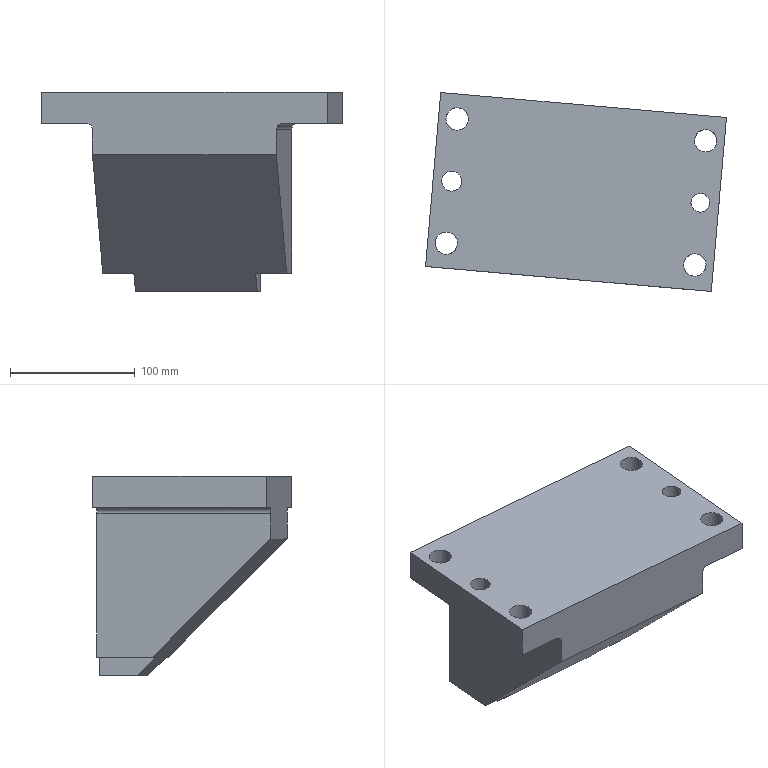Part | NX | features solid 2 | 1 solid | 31 faces | box 241.327 x 159.513 x 160 mm | volume 2643101 mm3 | plane 19 | cylinder 8 | spline 4 | commonest cylinder face diameters 18 x4 10 x2 15 x1 16 x1
STEP:
#1=CARTESIAN_POINT('',(296.017,170.851,90.));
#2=VERTEX_POINT('',#1);
#3=CARTESIAN_POINT('',(297.586,188.782,90.));
#4=VERTEX_POINT('',#3);
#5=CARTESIAN_POINT('',(296.017,170.851,90.));
#6=CARTESIAN_POINT('',(293.671,171.056,90.));
#7=CARTESIAN_POINT('',(289.163,173.405,90.));
#8=CARTESIAN_POINT('',(286.864,180.686,90.));
#9=CARTESIAN_POINT('',(290.394,187.456,90.));
#10=CARTESIAN_POINT('',(295.237,188.987,90.));
#11=CARTESIAN_POINT('',(297.586,188.782,90.));
#12=B_SPLINE_CURVE_WITH_KNOTS('',3,(#5,#6,#7,#8,#9,#10,#11),.UNSPECIFIED.,.F.,.F.,(4,1,1,1,4),(0.,0.125,0.25,0.375,0.5),.UNSPECIFIED.);
#13=EDGE_CURVE('',#2,#4,#12,.T.);
#14=ORIENTED_EDGE('',*,*,#13,.F.);
#15=CARTESIAN_POINT('',(297.586,188.782,90.));
#16=CARTESIAN_POINT('',(299.929,188.577,90.));
#17=CARTESIAN_POINT('',(304.441,186.227,90.));
#18=CARTESIAN_POINT('',(306.738,178.947,90.));
#19=CARTESIAN_POINT('',(303.211,172.176,90.));
#20=CARTESIAN_POINT('',(298.363,170.645,90.));
#21=CARTESIAN_POINT('',(296.017,170.851,90.));
#22=B_SPLINE_CURVE_WITH_KNOTS('',3,(#15,#16,#17,#18,#19,#20,#21),.UNSPECIFIED.,.F.,.F.,(4,1,1,1,4),(0.5,0.625,0.75,0.875,1.),.UNSPECIFIED.);
#23=EDGE_CURVE('',#4,#2,#22,.T.);
#24=ORIENTED_EDGE('',*,*,#23,.F.);
#25=EDGE_LOOP('',(#14,#24));
#26=FACE_BOUND('',#25,.T.);
#27=CARTESIAN_POINT('',(297.586,188.782,67.));
#28=VERTEX_POINT('',#27);
#29=CARTESIAN_POINT('',(296.801,179.816,67.));
#30=DIRECTION('',(0.,0.,-1.));
#31=DIRECTION('',(0.08716,0.9962,0.));
#32=AXIS2_PLACEMENT_3D('',#29,#30,#31);
#33=CIRCLE('',#32,9.);
#34=EDGE_CURVE('',#28,#28,#33,.F.);
#35=ORIENTED_EDGE('',*,*,#34,.F.);
#36=EDGE_LOOP('',(#35));
#37=FACE_BOUND('',#36,.T.);
#38=CARTESIAN_POINT('',(296.801,179.816,85.));
#39=DIRECTION('',(0.,0.,-1.));
#40=DIRECTION('',(0.9962,-0.08716,0.));
#41=AXIS2_PLACEMENT_3D('',#38,#39,#40);
#42=CYLINDRICAL_SURFACE('',#41,9.);
#43=ADVANCED_FACE('',(#26,#37),#42,.F.);
#44=CARTESIAN_POINT('',(304.733,270.47,90.));
#45=VERTEX_POINT('',#44);
#46=CARTESIAN_POINT('',(306.301,288.402,90.));
#47=VERTEX_POINT('',#46);
#48=CARTESIAN_POINT('',(304.733,270.47,90.));
#49=CARTESIAN_POINT('',(302.387,270.675,90.));
#50=CARTESIAN_POINT('',(297.879,273.025,90.));
#51=CARTESIAN_POINT('',(295.58,280.305,90.));
#52=CARTESIAN_POINT('',(299.109,287.076,90.));
#53=CARTESIAN_POINT('',(303.953,288.607,90.));
#54=CARTESIAN_POINT('',(306.301,288.402,90.));
#55=B_SPLINE_CURVE_WITH_KNOTS('',3,(#48,#49,#50,#51,#52,#53,#54),.UNSPECIFIED.,.F.,.F.,(4,1,1,1,4),(0.,0.125,0.25,0.375,0.5),.UNSPECIFIED.);
#56=EDGE_CURVE('',#45,#47,#55,.T.);
#57=ORIENTED_EDGE('',*,*,#56,.F.);
#58=CARTESIAN_POINT('',(306.301,288.402,90.));
#59=CARTESIAN_POINT('',(308.644,288.197,90.));
#60=CARTESIAN_POINT('',(313.157,285.847,90.));
#61=CARTESIAN_POINT('',(315.453,278.566,90.));
#62=CARTESIAN_POINT('',(311.926,271.796,90.));
#63=CARTESIAN_POINT('',(307.079,270.265,90.));
#64=CARTESIAN_POINT('',(304.733,270.47,90.));
#65=B_SPLINE_CURVE_WITH_KNOTS('',3,(#58,#59,#60,#61,#62,#63,#64),.UNSPECIFIED.,.F.,.F.,(4,1,1,1,4),(0.5,0.625,0.75,0.875,1.),.UNSPECIFIED.);
#66=EDGE_CURVE('',#47,#45,#65,.T.);
#67=ORIENTED_EDGE('',*,*,#66,.F.);
#68=EDGE_LOOP('',(#57,#67));
#69=FACE_BOUND('',#68,.T.);
#70=CARTESIAN_POINT('',(306.301,288.402,67.));
#71=VERTEX_POINT('',#70);
#72=CARTESIAN_POINT('',(305.517,279.436,67.));
#73=DIRECTION('',(0.,0.,-1.));
#74=DIRECTION('',(0.08716,0.9962,0.));
#75=AXIS2_PLACEMENT_3D('',#72,#73,#74);
#76=CIRCLE('',#75,9.);
#77=EDGE_CURVE('',#71,#71,#76,.F.);
#78=ORIENTED_EDGE('',*,*,#77,.F.);
#79=EDGE_LOOP('',(#78));
#80=FACE_BOUND('',#79,.T.);
#81=CARTESIAN_POINT('',(305.517,279.436,85.));
#82=DIRECTION('',(0.,0.,-1.));
#83=DIRECTION('',(0.9962,-0.08716,0.));
#84=AXIS2_PLACEMENT_3D('',#81,#82,#83);
#85=CYLINDRICAL_SURFACE('',#84,9.);
#86=ADVANCED_FACE('',(#69,#80),#85,.F.);
#87=CARTESIAN_POINT('',(495.256,153.419,90.));
#88=VERTEX_POINT('',#87);
#89=CARTESIAN_POINT('',(496.825,171.351,90.));
#90=VERTEX_POINT('',#89);
#91=CARTESIAN_POINT('',(495.256,153.419,90.));
#92=CARTESIAN_POINT('',(492.91,153.625,90.));
#93=CARTESIAN_POINT('',(488.402,155.974,90.));
#94=CARTESIAN_POINT('',(486.103,163.255,90.));
#95=CARTESIAN_POINT('',(489.633,170.025,90.));
#96=CARTESIAN_POINT('',(494.476,171.556,90.));
#97=CARTESIAN_POINT('',(496.825,171.351,90.));
#98=B_SPLINE_CURVE_WITH_KNOTS('',3,(#91,#92,#93,#94,#95,#96,#97),.UNSPECIFIED.,.F.,.F.,(4,1,1,1,4),(0.,0.125,0.25,0.375,0.5),.UNSPECIFIED.);
#99=EDGE_CURVE('',#88,#90,#98,.T.);
#100=ORIENTED_EDGE('',*,*,#99,.F.);
#101=CARTESIAN_POINT('',(496.825,171.351,90.));
#102=CARTESIAN_POINT('',(499.168,171.146,90.));
#103=CARTESIAN_POINT('',(503.68,168.796,90.));
#104=CARTESIAN_POINT('',(505.977,161.516,90.));
#105=CARTESIAN_POINT('',(502.449,154.745,90.));
#106=CARTESIAN_POINT('',(497.602,153.214,90.));
#107=CARTESIAN_POINT('',(495.256,153.419,90.));
#108=B_SPLINE_CURVE_WITH_KNOTS('',3,(#101,#102,#103,#104,#105,#106,#107),.UNSPECIFIED.,.F.,.F.,(4,1,1,1,4),(0.5,0.625,0.75,0.875,1.),.UNSPECIFIED.);
#109=EDGE_CURVE('',#90,#88,#108,.T.);
#110=ORIENTED_EDGE('',*,*,#109,.F.);
#111=EDGE_LOOP('',(#100,#110));
#112=FACE_BOUND('',#111,.T.);
#113=CARTESIAN_POINT('',(496.825,171.351,67.));
#114=VERTEX_POINT('',#113);
#115=CARTESIAN_POINT('',(496.04,162.385,67.));
#116=DIRECTION('',(0.,0.,-1.));
#117=DIRECTION('',(0.08716,0.9962,0.));
#118=AXIS2_PLACEMENT_3D('',#115,#116,#117);
#119=CIRCLE('',#118,9.);
#120=EDGE_CURVE('',#114,#114,#119,.F.);
#121=ORIENTED_EDGE('',*,*,#120,.F.);
#122=EDGE_LOOP('',(#121));
#123=FACE_BOUND('',#122,.T.);
#124=CARTESIAN_POINT('',(496.04,162.385,85.));
#125=DIRECTION('',(0.,0.,-1.));
#126=DIRECTION('',(0.9962,-0.08716,0.));
#127=AXIS2_PLACEMENT_3D('',#124,#125,#126);
#128=CYLINDRICAL_SURFACE('',#127,9.);
#129=ADVANCED_FACE('',(#112,#123),#128,.F.);
#130=CARTESIAN_POINT('',(503.972,253.039,90.));
#131=VERTEX_POINT('',#130);
#132=CARTESIAN_POINT('',(505.54,270.97,90.));
#133=VERTEX_POINT('',#132);
#134=CARTESIAN_POINT('',(503.972,253.039,90.));
#135=CARTESIAN_POINT('',(501.626,253.244,90.));
#136=CARTESIAN_POINT('',(497.118,255.593,90.));
#137=CARTESIAN_POINT('',(494.819,262.874,90.));
#138=CARTESIAN_POINT('',(498.348,269.645,90.));
#139=CARTESIAN_POINT('',(503.192,271.176,90.));
#140=CARTESIAN_POINT('',(505.54,270.97,90.));
#141=B_SPLINE_CURVE_WITH_KNOTS('',3,(#134,#135,#136,#137,#138,#139,#140),.UNSPECIFIED.,.F.,.F.,(4,1,1,1,4),(0.,0.125,0.25,0.375,0.5),.UNSPECIFIED.);
#142=EDGE_CURVE('',#131,#133,#141,.T.);
#143=ORIENTED_EDGE('',*,*,#142,.F.);
#144=CARTESIAN_POINT('',(505.54,270.97,90.));
#145=CARTESIAN_POINT('',(507.883,270.766,90.));
#146=CARTESIAN_POINT('',(512.396,268.416,90.));
#147=CARTESIAN_POINT('',(514.692,261.135,90.));
#148=CARTESIAN_POINT('',(511.165,254.365,90.));
#149=CARTESIAN_POINT('',(506.317,252.833,90.));
#150=CARTESIAN_POINT('',(503.972,253.039,90.));
#151=B_SPLINE_CURVE_WITH_KNOTS('',3,(#144,#145,#146,#147,#148,#149,#150),.UNSPECIFIED.,.F.,.F.,(4,1,1,1,4),(0.5,0.625,0.75,0.875,1.),.UNSPECIFIED.);
#152=EDGE_CURVE('',#133,#131,#151,.T.);
#153=ORIENTED_EDGE('',*,*,#152,.F.);
#154=EDGE_LOOP('',(#143,#153));
#155=FACE_BOUND('',#154,.T.);
#156=CARTESIAN_POINT('',(505.54,270.97,67.));
#157=VERTEX_POINT('',#156);
#158=CARTESIAN_POINT('',(504.756,262.005,67.));
#159=DIRECTION('',(0.,0.,-1.));
#160=DIRECTION('',(0.08716,0.9962,0.));
#161=AXIS2_PLACEMENT_3D('',#158,#159,#160);
#162=CIRCLE('',#161,9.);
#163=EDGE_CURVE('',#157,#157,#162,.F.);
#164=ORIENTED_EDGE('',*,*,#163,.F.);
#165=EDGE_LOOP('',(#164));
#166=FACE_BOUND('',#165,.T.);
#167=CARTESIAN_POINT('',(504.756,262.005,85.));
#168=DIRECTION('',(0.,0.,-1.));
#169=DIRECTION('',(0.9962,-0.08716,0.));
#170=AXIS2_PLACEMENT_3D('',#167,#168,#169);
#171=CYLINDRICAL_SURFACE('',#170,9.);
#172=ADVANCED_FACE('',(#155,#166),#171,.F.);
#173=ORIENTED_EDGE('',*,*,#23,.T.);
#174=ORIENTED_EDGE('',*,*,#13,.T.);
#175=EDGE_LOOP('',(#173,#174));
#176=FACE_BOUND('',#175,.T.);
#177=ORIENTED_EDGE('',*,*,#152,.T.);
#178=ORIENTED_EDGE('',*,*,#142,.T.);
#179=EDGE_LOOP('',(#177,#178));
#180=FACE_BOUND('',#179,.T.);
#181=CARTESIAN_POINT('',(501.052,219.666,90.));
#182=VERTEX_POINT('',#181);
#183=CARTESIAN_POINT('',(499.745,204.723,90.));
#184=VERTEX_POINT('',#183);
#185=CARTESIAN_POINT('',(501.052,219.666,90.));
#186=CARTESIAN_POINT('',(503.004,219.496,90.));
#187=CARTESIAN_POINT('',(506.765,217.537,90.));
#188=CARTESIAN_POINT('',(508.678,211.47,90.));
#189=CARTESIAN_POINT('',(505.739,205.828,90.));
#190=CARTESIAN_POINT('',(501.699,204.552,90.));
#191=CARTESIAN_POINT('',(499.745,204.723,90.));
#192=B_SPLINE_CURVE_WITH_KNOTS('',3,(#185,#186,#187,#188,#189,#190,#191),.UNSPECIFIED.,.F.,.F.,(4,1,1,1,4),(0.5,0.625,0.75,0.875,1.),.UNSPECIFIED.);
#193=EDGE_CURVE('',#182,#184,#192,.T.);
#194=ORIENTED_EDGE('',*,*,#193,.T.);
#195=CARTESIAN_POINT('',(499.745,204.723,90.));
#196=CARTESIAN_POINT('',(497.79,204.895,90.));
#197=CARTESIAN_POINT('',(494.033,206.852,90.));
#198=CARTESIAN_POINT('',(492.117,212.919,90.));
#199=CARTESIAN_POINT('',(495.059,218.562,90.));
#200=CARTESIAN_POINT('',(499.094,219.837,90.));
#201=CARTESIAN_POINT('',(501.052,219.666,90.));
#202=B_SPLINE_CURVE_WITH_KNOTS('',3,(#195,#196,#197,#198,#199,#200,#201),.UNSPECIFIED.,.F.,.F.,(4,1,1,1,4),(0.,0.125,0.25,0.375,0.5),.UNSPECIFIED.);
#203=EDGE_CURVE('',#184,#182,#202,.T.);
#204=ORIENTED_EDGE('',*,*,#203,.T.);
#205=EDGE_LOOP('',(#194,#204));
#206=FACE_BOUND('',#205,.T.);
#207=CARTESIAN_POINT('',(301.856,237.596,90.));
#208=VERTEX_POINT('',#207);
#209=CARTESIAN_POINT('',(300.462,221.656,90.));
#210=VERTEX_POINT('',#209);
#211=CARTESIAN_POINT('',(301.159,229.626,90.));
#212=DIRECTION('',(0.,0.,1.));
#213=DIRECTION('',(0.08716,0.9962,0.));
#214=AXIS2_PLACEMENT_3D('',#211,#212,#213);
#215=CIRCLE('',#214,8.);
#216=EDGE_CURVE('',#208,#210,#215,.F.);
#217=ORIENTED_EDGE('',*,*,#216,.T.);
#218=CARTESIAN_POINT('',(301.159,229.626,90.));
#219=DIRECTION('',(0.,0.,1.));
#220=DIRECTION('',(0.08716,0.9962,0.));
#221=AXIS2_PLACEMENT_3D('',#218,#219,#220);
#222=CIRCLE('',#221,8.);
#223=EDGE_CURVE('',#210,#208,#222,.F.);
#224=ORIENTED_EDGE('',*,*,#223,.T.);
#225=EDGE_LOOP('',(#217,#224));
#226=FACE_BOUND('',#225,.T.);
#227=ORIENTED_EDGE('',*,*,#109,.T.);
#228=ORIENTED_EDGE('',*,*,#99,.T.);
#229=EDGE_LOOP('',(#227,#228));
#230=FACE_BOUND('',#229,.T.);
#231=ORIENTED_EDGE('',*,*,#66,.T.);
#232=ORIENTED_EDGE('',*,*,#56,.T.);
#233=EDGE_LOOP('',(#231,#232));
#234=FACE_BOUND('',#233,.T.);
#235=CARTESIAN_POINT('',(292.317,300.667,90.));
#236=VERTEX_POINT('',#235);
#237=CARTESIAN_POINT('',(280.115,161.2,90.));
#238=VERTEX_POINT('',#237);
#239=CARTESIAN_POINT('',(292.317,300.667,90.));
#240=CARTESIAN_POINT('',(288.25,254.178,90.));
#241=CARTESIAN_POINT('',(284.183,207.689,90.));
#242=CARTESIAN_POINT('',(280.115,161.2,90.));
#243=B_SPLINE_CURVE_WITH_KNOTS('',3,(#239,#240,#241,#242),.UNSPECIFIED.,.F.,.F.,(4,4),(0.,1.),.UNSPECIFIED.);
#244=EDGE_CURVE('',#236,#238,#243,.T.);
#245=ORIENTED_EDGE('',*,*,#244,.T.);
#246=CARTESIAN_POINT('',(509.24,141.154,90.));
#247=VERTEX_POINT('',#246);
#248=CARTESIAN_POINT('',(280.115,161.2,90.));
#249=CARTESIAN_POINT('',(356.49,154.518,90.));
#250=CARTESIAN_POINT('',(432.865,147.836,90.));
#251=CARTESIAN_POINT('',(509.24,141.154,90.));
#252=B_SPLINE_CURVE_WITH_KNOTS('',3,(#248,#249,#250,#251),.UNSPECIFIED.,.F.,.F.,(4,4),(0.,1.),.UNSPECIFIED.);
#253=EDGE_CURVE('',#238,#247,#252,.T.);
#254=ORIENTED_EDGE('',*,*,#253,.T.);
#255=CARTESIAN_POINT('',(521.442,280.621,90.));
#256=VERTEX_POINT('',#255);
#257=CARTESIAN_POINT('',(509.24,141.154,90.));
#258=CARTESIAN_POINT('',(513.307,187.643,90.));
#259=CARTESIAN_POINT('',(517.375,234.132,90.));
#260=CARTESIAN_POINT('',(521.442,280.621,90.));
#261=B_SPLINE_CURVE_WITH_KNOTS('',3,(#257,#258,#259,#260),.UNSPECIFIED.,.F.,.F.,(4,4),(0.,1.),.UNSPECIFIED.);
#262=EDGE_CURVE('',#247,#256,#261,.T.);
#263=ORIENTED_EDGE('',*,*,#262,.T.);
#264=CARTESIAN_POINT('',(521.442,280.621,90.));
#265=CARTESIAN_POINT('',(445.067,287.303,90.));
#266=CARTESIAN_POINT('',(368.692,293.985,90.));
#267=CARTESIAN_POINT('',(292.317,300.667,90.));
#268=B_SPLINE_CURVE_WITH_KNOTS('',3,(#264,#265,#266,#267),.UNSPECIFIED.,.F.,.F.,(4,4),(0.,1.),.UNSPECIFIED.);
#269=EDGE_CURVE('',#256,#236,#268,.T.);
#270=ORIENTED_EDGE('',*,*,#269,.T.);
#271=EDGE_LOOP('',(#245,#254,#263,#270));
#272=FACE_BOUND('',#271,.T.);
#273=CARTESIAN_POINT('',(400.779,220.91,90.));
#274=DIRECTION('',(0.,0.,1.));
#275=DIRECTION('',(0.08716,0.9962,0.));
#276=AXIS2_PLACEMENT_3D('',#273,#274,#275);
#277=PLANE('',#276);
#278=ADVANCED_FACE('',(#176,#180,#206,#226,#230,#234,#272),#277,.T.);
#279=CARTESIAN_POINT('',(501.052,219.666,65.));
#280=VERTEX_POINT('',#279);
#281=CARTESIAN_POINT('',(499.745,204.723,65.));
#282=VERTEX_POINT('',#281);
#283=CARTESIAN_POINT('',(499.745,204.723,65.));
#284=CARTESIAN_POINT('',(501.697,204.553,65.));
#285=CARTESIAN_POINT('',(505.74,205.828,65.));
#286=CARTESIAN_POINT('',(508.678,211.47,65.));
#287=CARTESIAN_POINT('',(506.764,217.537,65.));
#288=CARTESIAN_POINT('',(503.007,219.495,65.));
#289=CARTESIAN_POINT('',(501.052,219.666,65.));
#290=B_SPLINE_CURVE_WITH_KNOTS('',3,(#283,#284,#285,#286,#287,#288,#289),.UNSPECIFIED.,.F.,.F.,(4,1,1,1,4),(0.5,0.625,0.75,0.875,1.),.UNSPECIFIED.);
#291=EDGE_CURVE('',#280,#282,#290,.F.);
#292=ORIENTED_EDGE('',*,*,#291,.T.);
#293=CARTESIAN_POINT('',(501.052,219.666,65.));
#294=CARTESIAN_POINT('',(499.097,219.837,65.));
#295=CARTESIAN_POINT('',(495.057,218.562,65.));
#296=CARTESIAN_POINT('',(492.117,212.919,65.));
#297=CARTESIAN_POINT('',(494.034,206.852,65.));
#298=CARTESIAN_POINT('',(497.787,204.895,65.));
#299=CARTESIAN_POINT('',(499.745,204.723,65.));
#300=B_SPLINE_CURVE_WITH_KNOTS('',3,(#293,#294,#295,#296,#297,#298,#299),.UNSPECIFIED.,.F.,.F.,(4,1,1,1,4),(0.,0.125,0.25,0.375,0.5),.UNSPECIFIED.);
#301=EDGE_CURVE('',#282,#280,#300,.F.);
#302=ORIENTED_EDGE('',*,*,#301,.T.);
#303=EDGE_LOOP('',(#292,#302));
#304=FACE_BOUND('',#303,.T.);
#305=ORIENTED_EDGE('',*,*,#203,.F.);
#306=ORIENTED_EDGE('',*,*,#193,.F.);
#307=EDGE_LOOP('',(#305,#306));
#308=FACE_BOUND('',#307,.T.);
#309=CARTESIAN_POINT('',(500.398,212.195,85.));
#310=DIRECTION('',(0.,0.,-1.));
#311=DIRECTION('',(0.9962,-0.08716,0.));
#312=AXIS2_PLACEMENT_3D('',#309,#310,#311);
#313=CYLINDRICAL_SURFACE('',#312,7.5);
#314=ADVANCED_FACE('',(#304,#308),#313,.F.);
#315=CARTESIAN_POINT('',(301.856,237.596,65.));
#316=VERTEX_POINT('',#315);
#317=CARTESIAN_POINT('',(300.462,221.656,65.));
#318=VERTEX_POINT('',#317);
#319=CARTESIAN_POINT('',(301.159,229.626,65.));
#320=DIRECTION('',(0.,0.,-1.));
#321=DIRECTION('',(0.9962,-0.08716,0.));
#322=AXIS2_PLACEMENT_3D('',#319,#320,#321);
#323=CIRCLE('',#322,8.);
#324=EDGE_CURVE('',#316,#318,#323,.T.);
#325=ORIENTED_EDGE('',*,*,#324,.T.);
#326=CARTESIAN_POINT('',(301.159,229.626,65.));
#327=DIRECTION('',(0.,0.,-1.));
#328=DIRECTION('',(0.9962,-0.08716,0.));
#329=AXIS2_PLACEMENT_3D('',#326,#327,#328);
#330=CIRCLE('',#329,8.);
#331=EDGE_CURVE('',#318,#316,#330,.T.);
#332=ORIENTED_EDGE('',*,*,#331,.T.);
#333=EDGE_LOOP('',(#325,#332));
#334=FACE_BOUND('',#333,.T.);
#335=ORIENTED_EDGE('',*,*,#223,.F.);
#336=ORIENTED_EDGE('',*,*,#216,.F.);
#337=EDGE_LOOP('',(#335,#336));
#338=FACE_BOUND('',#337,.T.);
#339=CARTESIAN_POINT('',(301.159,229.626,85.));
#340=DIRECTION('',(0.,0.,-1.));
#341=DIRECTION('',(0.9962,-0.08716,0.));
#342=AXIS2_PLACEMENT_3D('',#339,#340,#341);
#343=CYLINDRICAL_SURFACE('',#342,8.);
#344=ADVANCED_FACE('',(#334,#338),#343,.F.);
#345=CARTESIAN_POINT('',(280.115,161.2,65.));
#346=VERTEX_POINT('',#345);
#347=CARTESIAN_POINT('',(315.978,158.062,65.));
#348=VERTEX_POINT('',#347);
#349=CARTESIAN_POINT('',(280.115,161.2,65.));
#350=CARTESIAN_POINT('',(292.07,160.154,65.));
#351=CARTESIAN_POINT('',(304.024,159.108,65.));
#352=CARTESIAN_POINT('',(315.978,158.062,65.));
#353=B_SPLINE_CURVE_WITH_KNOTS('',3,(#349,#350,#351,#352),.UNSPECIFIED.,.F.,.F.,(4,4),(0.,1.),.UNSPECIFIED.);
#354=EDGE_CURVE('',#346,#348,#353,.T.);
#355=ORIENTED_EDGE('',*,*,#354,.T.);
#356=CARTESIAN_POINT('',(320.959,157.626,60.));
#357=VERTEX_POINT('',#356);
#358=CARTESIAN_POINT('',(315.978,158.062,65.));
#359=CARTESIAN_POINT('',(316.086,158.053,64.999));
#360=CARTESIAN_POINT('',(316.211,158.042,64.997));
#361=CARTESIAN_POINT('',(316.554,158.012,64.972));
#362=CARTESIAN_POINT('',(317.107,157.963,64.888));
#363=CARTESIAN_POINT('',(317.897,157.894,64.65));
#364=CARTESIAN_POINT('',(318.76,157.819,64.186));
#365=CARTESIAN_POINT('',(319.523,157.752,63.559));
#366=CARTESIAN_POINT('',(320.148,157.697,62.793));
#367=CARTESIAN_POINT('',(320.611,157.657,61.926));
#368=CARTESIAN_POINT('',(320.846,157.636,61.133));
#369=CARTESIAN_POINT('',(320.933,157.629,60.579));
#370=CARTESIAN_POINT('',(320.954,157.627,60.233));
#371=CARTESIAN_POINT('',(320.957,157.627,60.109));
#372=CARTESIAN_POINT('',(320.959,157.626,60.));
#373=B_SPLINE_CURVE_WITH_KNOTS('',3,(#358,#359,#360,#361,#362,#363,#364,#365,#366,#367,#368,#369,#370,#371,#372),.UNSPECIFIED.,.F.,.F.,(4,1,1,1,1,1,1,1,1,1,1,1,4),(0.,0.03125,0.0625,0.125,0.25,0.375,0.5,0.625,0.75,0.875,0.9375,0.9688,1.),.UNSPECIFIED.);
#374=EDGE_CURVE('',#348,#357,#373,.T.);
#375=ORIENTED_EDGE('',*,*,#374,.T.);
#376=CARTESIAN_POINT('',(320.959,157.626,40.));
#377=VERTEX_POINT('',#376);
#378=CARTESIAN_POINT('',(320.959,157.626,60.));
#379=CARTESIAN_POINT('',(320.959,157.626,53.333));
#380=CARTESIAN_POINT('',(320.959,157.626,46.667));
#381=CARTESIAN_POINT('',(320.959,157.626,40.));
#382=B_SPLINE_CURVE_WITH_KNOTS('',3,(#378,#379,#380,#381),.UNSPECIFIED.,.F.,.F.,(4,4),(0.,1.),.UNSPECIFIED.);
#383=EDGE_CURVE('',#357,#377,#382,.T.);
#384=ORIENTED_EDGE('',*,*,#383,.T.);
#385=CARTESIAN_POINT('',(468.396,144.727,40.));
#386=VERTEX_POINT('',#385);
#387=CARTESIAN_POINT('',(320.959,157.626,40.));
#388=CARTESIAN_POINT('',(370.105,153.327,40.));
#389=CARTESIAN_POINT('',(419.251,149.027,40.));
#390=CARTESIAN_POINT('',(468.396,144.727,40.));
#391=B_SPLINE_CURVE_WITH_KNOTS('',3,(#387,#388,#389,#390),.UNSPECIFIED.,.F.,.F.,(4,4),(0.,1.),.UNSPECIFIED.);
#392=EDGE_CURVE('',#377,#386,#391,.T.);
#393=ORIENTED_EDGE('',*,*,#392,.T.);
#394=CARTESIAN_POINT('',(468.396,144.727,60.));
#395=VERTEX_POINT('',#394);
#396=CARTESIAN_POINT('',(468.396,144.727,40.));
#397=CARTESIAN_POINT('',(468.396,144.727,46.667));
#398=CARTESIAN_POINT('',(468.396,144.727,53.333));
#399=CARTESIAN_POINT('',(468.396,144.727,60.));
#400=B_SPLINE_CURVE_WITH_KNOTS('',3,(#396,#397,#398,#399),.UNSPECIFIED.,.F.,.F.,(4,4),(0.,1.),.UNSPECIFIED.);
#401=EDGE_CURVE('',#386,#395,#400,.T.);
#402=ORIENTED_EDGE('',*,*,#401,.T.);
#403=CARTESIAN_POINT('',(473.377,144.292,65.));
#404=VERTEX_POINT('',#403);
#405=CARTESIAN_POINT('',(468.396,144.727,60.));
#406=CARTESIAN_POINT('',(468.398,144.727,60.108));
#407=CARTESIAN_POINT('',(468.399,144.727,60.233));
#408=CARTESIAN_POINT('',(468.424,144.725,60.578));
#409=CARTESIAN_POINT('',(468.507,144.718,61.133));
#410=CARTESIAN_POINT('',(468.745,144.697,61.926));
#411=CARTESIAN_POINT('',(469.207,144.656,62.792));
#412=CARTESIAN_POINT('',(469.832,144.602,63.559));
#413=CARTESIAN_POINT('',(470.595,144.535,64.185));
#414=CARTESIAN_POINT('',(471.458,144.459,64.65));
#415=CARTESIAN_POINT('',(472.248,144.39,64.887));
#416=CARTESIAN_POINT('',(472.801,144.342,64.974));
#417=CARTESIAN_POINT('',(473.145,144.312,64.994));
#418=CARTESIAN_POINT('',(473.268,144.301,64.997));
#419=CARTESIAN_POINT('',(473.377,144.292,65.));
#420=B_SPLINE_CURVE_WITH_KNOTS('',3,(#405,#406,#407,#408,#409,#410,#411,#412,#413,#414,#415,#416,#417,#418,#419),.UNSPECIFIED.,.F.,.F.,(4,1,1,1,1,1,1,1,1,1,1,1,4),(0.,0.03125,0.0625,0.125,0.25,0.375,0.5,0.625,0.75,0.875,0.9375,0.9688,1.),.UNSPECIFIED.);
#421=EDGE_CURVE('',#395,#404,#420,.T.);
#422=ORIENTED_EDGE('',*,*,#421,.T.);
#423=CARTESIAN_POINT('',(509.24,141.154,65.));
#424=VERTEX_POINT('',#423);
#425=CARTESIAN_POINT('',(473.377,144.292,65.));
#426=CARTESIAN_POINT('',(485.332,143.246,65.));
#427=CARTESIAN_POINT('',(497.286,142.2,65.));
#428=CARTESIAN_POINT('',(509.24,141.154,65.));
#429=B_SPLINE_CURVE_WITH_KNOTS('',3,(#425,#426,#427,#428),.UNSPECIFIED.,.F.,.F.,(4,4),(0.,1.),.UNSPECIFIED.);
#430=EDGE_CURVE('',#404,#424,#429,.T.);
#431=ORIENTED_EDGE('',*,*,#430,.T.);
#432=CARTESIAN_POINT('',(509.24,141.154,65.));
#433=CARTESIAN_POINT('',(509.24,141.154,73.333));
#434=CARTESIAN_POINT('',(509.24,141.154,81.667));
#435=CARTESIAN_POINT('',(509.24,141.154,90.));
#436=B_SPLINE_CURVE_WITH_KNOTS('',3,(#432,#433,#434,#435),.UNSPECIFIED.,.F.,.F.,(4,4),(0.,1.),.UNSPECIFIED.);
#437=EDGE_CURVE('',#424,#247,#436,.T.);
#438=ORIENTED_EDGE('',*,*,#437,.T.);
#439=ORIENTED_EDGE('',*,*,#253,.F.);
#440=CARTESIAN_POINT('',(280.115,161.2,90.));
#441=CARTESIAN_POINT('',(280.115,161.2,81.667));
#442=CARTESIAN_POINT('',(280.115,161.2,73.333));
#443=CARTESIAN_POINT('',(280.115,161.2,65.));
#444=B_SPLINE_CURVE_WITH_KNOTS('',3,(#440,#441,#442,#443),.UNSPECIFIED.,.F.,.F.,(4,4),(0.,1.),.UNSPECIFIED.);
#445=EDGE_CURVE('',#238,#346,#444,.T.);
#446=ORIENTED_EDGE('',*,*,#445,.T.);
#447=EDGE_LOOP('',(#355,#375,#384,#393,#402,#422,#431,#438,#439,#446));
#448=FACE_BOUND('',#447,.T.);
#449=CARTESIAN_POINT('',(394.678,151.177,65.));
#450=DIRECTION('',(-0.08716,-0.9962,0.));
#451=DIRECTION('',(0.9962,-0.08716,0.));
#452=AXIS2_PLACEMENT_3D('',#449,#450,#451);
#453=PLANE('',#452);
#454=ADVANCED_FACE('',(#448),#453,.T.);
#455=ORIENTED_EDGE('',*,*,#244,.F.);
#456=CARTESIAN_POINT('',(292.317,300.667,65.));
#457=VERTEX_POINT('',#456);
#458=CARTESIAN_POINT('',(292.317,300.667,90.));
#459=CARTESIAN_POINT('',(292.317,300.667,81.667));
#460=CARTESIAN_POINT('',(292.317,300.667,73.333));
#461=CARTESIAN_POINT('',(292.317,300.667,65.));
#462=B_SPLINE_CURVE_WITH_KNOTS('',3,(#458,#459,#460,#461),.UNSPECIFIED.,.F.,.F.,(4,4),(0.,1.),.UNSPECIFIED.);
#463=EDGE_CURVE('',#236,#457,#462,.T.);
#464=ORIENTED_EDGE('',*,*,#463,.T.);
#465=CARTESIAN_POINT('',(292.317,300.667,65.));
#466=CARTESIAN_POINT('',(288.25,254.178,65.));
#467=CARTESIAN_POINT('',(284.183,207.689,65.));
#468=CARTESIAN_POINT('',(280.115,161.2,65.));
#469=B_SPLINE_CURVE_WITH_KNOTS('',3,(#465,#466,#467,#468),.UNSPECIFIED.,.F.,.F.,(4,4),(0.,1.),.UNSPECIFIED.);
#470=EDGE_CURVE('',#457,#346,#469,.T.);
#471=ORIENTED_EDGE('',*,*,#470,.T.);
#472=ORIENTED_EDGE('',*,*,#445,.F.);
#473=EDGE_LOOP('',(#455,#464,#471,#472));
#474=FACE_BOUND('',#473,.T.);
#475=CARTESIAN_POINT('',(286.216,230.933,77.5));
#476=DIRECTION('',(-0.9962,0.08716,0.));
#477=DIRECTION('',(-0.08716,-0.9962,0.));
#478=AXIS2_PLACEMENT_3D('',#475,#476,#477);
#479=PLANE('',#478);
#480=ADVANCED_FACE('',(#474),#479,.T.);
#481=CARTESIAN_POINT('',(455.693,286.373,-55.));
#482=VERTEX_POINT('',#481);
#483=CARTESIAN_POINT('',(455.693,286.373,-70.));
#484=VERTEX_POINT('',#483);
#485=CARTESIAN_POINT('',(455.693,286.373,-55.));
#486=CARTESIAN_POINT('',(455.693,286.373,-60.));
#487=CARTESIAN_POINT('',(455.693,286.373,-65.));
#488=CARTESIAN_POINT('',(455.693,286.373,-70.));
#489=B_SPLINE_CURVE_WITH_KNOTS('',3,(#485,#486,#487,#488),.UNSPECIFIED.,.F.,.F.,(4,4),(0.,1.),.UNSPECIFIED.);
#490=EDGE_CURVE('',#482,#484,#489,.T.);
#491=ORIENTED_EDGE('',*,*,#490,.T.);
#492=CARTESIAN_POINT('',(358.066,294.915,-70.));
#493=VERTEX_POINT('',#492);
#494=CARTESIAN_POINT('',(455.693,286.373,-70.));
#495=CARTESIAN_POINT('',(423.151,289.221,-70.));
#496=CARTESIAN_POINT('',(390.608,292.068,-70.));
#497=CARTESIAN_POINT('',(358.066,294.915,-70.));
#498=B_SPLINE_CURVE_WITH_KNOTS('',3,(#494,#495,#496,#497),.UNSPECIFIED.,.F.,.F.,(4,4),(0.,1.),.UNSPECIFIED.);
#499=EDGE_CURVE('',#484,#493,#498,.T.);
#500=ORIENTED_EDGE('',*,*,#499,.T.);
#501=CARTESIAN_POINT('',(358.066,294.915,-55.));
#502=VERTEX_POINT('',#501);
#503=CARTESIAN_POINT('',(358.066,294.915,-70.));
#504=CARTESIAN_POINT('',(358.066,294.915,-65.));
#505=CARTESIAN_POINT('',(358.066,294.915,-60.));
#506=CARTESIAN_POINT('',(358.066,294.915,-55.));
#507=B_SPLINE_CURVE_WITH_KNOTS('',3,(#503,#504,#505,#506),.UNSPECIFIED.,.F.,.F.,(4,4),(0.,1.),.UNSPECIFIED.);
#508=EDGE_CURVE('',#493,#502,#507,.T.);
#509=ORIENTED_EDGE('',*,*,#508,.T.);
#510=CARTESIAN_POINT('',(333.161,297.094,-55.));
#511=VERTEX_POINT('',#510);
#512=CARTESIAN_POINT('',(358.066,294.915,-55.));
#513=CARTESIAN_POINT('',(349.764,295.641,-55.));
#514=CARTESIAN_POINT('',(341.463,296.367,-55.));
#515=CARTESIAN_POINT('',(333.161,297.094,-55.));
#516=B_SPLINE_CURVE_WITH_KNOTS('',3,(#512,#513,#514,#515),.UNSPECIFIED.,.F.,.F.,(4,4),(0.,1.),.UNSPECIFIED.);
#517=EDGE_CURVE('',#502,#511,#516,.T.);
#518=ORIENTED_EDGE('',*,*,#517,.T.);
#519=CARTESIAN_POINT('',(333.161,297.094,60.));
#520=VERTEX_POINT('',#519);
#521=CARTESIAN_POINT('',(333.161,297.094,-55.));
#522=CARTESIAN_POINT('',(333.161,297.094,-16.667));
#523=CARTESIAN_POINT('',(333.161,297.094,21.667));
#524=CARTESIAN_POINT('',(333.161,297.094,60.));
#525=B_SPLINE_CURVE_WITH_KNOTS('',3,(#521,#522,#523,#524),.UNSPECIFIED.,.F.,.F.,(4,4),(0.,1.),.UNSPECIFIED.);
#526=EDGE_CURVE('',#511,#520,#525,.T.);
#527=ORIENTED_EDGE('',*,*,#526,.T.);
#528=CARTESIAN_POINT('',(328.18,297.529,65.));
#529=VERTEX_POINT('',#528);
#530=CARTESIAN_POINT('',(333.161,297.094,60.));
#531=CARTESIAN_POINT('',(333.16,297.094,60.108));
#532=CARTESIAN_POINT('',(333.158,297.094,60.233));
#533=CARTESIAN_POINT('',(333.133,297.096,60.578));
#534=CARTESIAN_POINT('',(333.05,297.103,61.133));
#535=CARTESIAN_POINT('',(332.813,297.124,61.926));
#536=CARTESIAN_POINT('',(332.35,297.165,62.792));
#537=CARTESIAN_POINT('',(331.726,297.219,63.559));
#538=CARTESIAN_POINT('',(330.963,297.286,64.185));
#539=CARTESIAN_POINT('',(330.099,297.362,64.65));
#540=CARTESIAN_POINT('',(329.309,297.431,64.887));
#541=CARTESIAN_POINT('',(328.757,297.479,64.974));
#542=CARTESIAN_POINT('',(328.412,297.509,64.994));
#543=CARTESIAN_POINT('',(328.289,297.52,64.997));
#544=CARTESIAN_POINT('',(328.18,297.529,65.));
#545=B_SPLINE_CURVE_WITH_KNOTS('',3,(#530,#531,#532,#533,#534,#535,#536,#537,#538,#539,#540,#541,#542,#543,#544),.UNSPECIFIED.,.F.,.F.,(4,1,1,1,1,1,1,1,1,1,1,1,4),(0.,0.03125,0.0625,0.125,0.25,0.375,0.5,0.625,0.75,0.875,0.9375,0.9688,1.),.UNSPECIFIED.);
#546=EDGE_CURVE('',#520,#529,#545,.T.);
#547=ORIENTED_EDGE('',*,*,#546,.T.);
#548=CARTESIAN_POINT('',(328.18,297.529,65.));
#549=CARTESIAN_POINT('',(316.226,298.575,65.));
#550=CARTESIAN_POINT('',(304.272,299.621,65.));
#551=CARTESIAN_POINT('',(292.317,300.667,65.));
#552=B_SPLINE_CURVE_WITH_KNOTS('',3,(#548,#549,#550,#551),.UNSPECIFIED.,.F.,.F.,(4,4),(0.,1.),.UNSPECIFIED.);
#553=EDGE_CURVE('',#529,#457,#552,.T.);
#554=ORIENTED_EDGE('',*,*,#553,.T.);
#555=ORIENTED_EDGE('',*,*,#463,.F.);
#556=ORIENTED_EDGE('',*,*,#269,.F.);
#557=CARTESIAN_POINT('',(521.442,280.621,65.));
#558=VERTEX_POINT('',#557);
#559=CARTESIAN_POINT('',(521.442,280.621,90.));
#560=CARTESIAN_POINT('',(521.442,280.621,81.667));
#561=CARTESIAN_POINT('',(521.442,280.621,73.333));
#562=CARTESIAN_POINT('',(521.442,280.621,65.));
#563=B_SPLINE_CURVE_WITH_KNOTS('',3,(#559,#560,#561,#562),.UNSPECIFIED.,.F.,.F.,(4,4),(0.,1.),.UNSPECIFIED.);
#564=EDGE_CURVE('',#256,#558,#563,.T.);
#565=ORIENTED_EDGE('',*,*,#564,.T.);
#566=CARTESIAN_POINT('',(485.579,283.759,65.));
#567=VERTEX_POINT('',#566);
#568=CARTESIAN_POINT('',(521.442,280.621,65.));
#569=CARTESIAN_POINT('',(509.488,281.667,65.));
#570=CARTESIAN_POINT('',(497.533,282.713,65.));
#571=CARTESIAN_POINT('',(485.579,283.759,65.));
#572=B_SPLINE_CURVE_WITH_KNOTS('',3,(#568,#569,#570,#571),.UNSPECIFIED.,.F.,.F.,(4,4),(0.,1.),.UNSPECIFIED.);
#573=EDGE_CURVE('',#558,#567,#572,.T.);
#574=ORIENTED_EDGE('',*,*,#573,.T.);
#575=CARTESIAN_POINT('',(480.598,284.195,60.));
#576=VERTEX_POINT('',#575);
#577=CARTESIAN_POINT('',(485.579,283.759,65.));
#578=CARTESIAN_POINT('',(485.471,283.768,64.999));
#579=CARTESIAN_POINT('',(485.347,283.779,64.997));
#580=CARTESIAN_POINT('',(485.003,283.809,64.972));
#581=CARTESIAN_POINT('',(484.45,283.858,64.888));
#582=CARTESIAN_POINT('',(483.661,283.927,64.65));
#583=CARTESIAN_POINT('',(482.797,284.002,64.186));
#584=CARTESIAN_POINT('',(482.034,284.069,63.559));
#585=CARTESIAN_POINT('',(481.41,284.124,62.793));
#586=CARTESIAN_POINT('',(480.946,284.164,61.926));
#587=CARTESIAN_POINT('',(480.711,284.185,61.133));
#588=CARTESIAN_POINT('',(480.624,284.192,60.579));
#589=CARTESIAN_POINT('',(480.604,284.194,60.233));
#590=CARTESIAN_POINT('',(480.601,284.194,60.109));
#591=CARTESIAN_POINT('',(480.598,284.195,60.));
#592=B_SPLINE_CURVE_WITH_KNOTS('',3,(#577,#578,#579,#580,#581,#582,#583,#584,#585,#586,#587,#588,#589,#590,#591),.UNSPECIFIED.,.F.,.F.,(4,1,1,1,1,1,1,1,1,1,1,1,4),(0.,0.03125,0.0625,0.125,0.25,0.375,0.5,0.625,0.75,0.875,0.9375,0.9688,1.),.UNSPECIFIED.);
#593=EDGE_CURVE('',#567,#576,#592,.T.);
#594=ORIENTED_EDGE('',*,*,#593,.T.);
#595=CARTESIAN_POINT('',(480.598,284.195,-55.));
#596=VERTEX_POINT('',#595);
#597=CARTESIAN_POINT('',(480.598,284.195,60.));
#598=CARTESIAN_POINT('',(480.598,284.195,21.667));
#599=CARTESIAN_POINT('',(480.598,284.195,-16.667));
#600=CARTESIAN_POINT('',(480.598,284.195,-55.));
#601=B_SPLINE_CURVE_WITH_KNOTS('',3,(#597,#598,#599,#600),.UNSPECIFIED.,.F.,.F.,(4,4),(0.,1.),.UNSPECIFIED.);
#602=EDGE_CURVE('',#576,#596,#601,.T.);
#603=ORIENTED_EDGE('',*,*,#602,.T.);
#604=CARTESIAN_POINT('',(480.598,284.195,-55.));
#605=CARTESIAN_POINT('',(472.296,284.921,-55.));
#606=CARTESIAN_POINT('',(463.995,285.647,-55.));
#607=CARTESIAN_POINT('',(455.693,286.373,-55.));
#608=B_SPLINE_CURVE_WITH_KNOTS('',3,(#604,#605,#606,#607),.UNSPECIFIED.,.F.,.F.,(4,4),(0.,1.),.UNSPECIFIED.);
#609=EDGE_CURVE('',#596,#482,#608,.T.);
#610=ORIENTED_EDGE('',*,*,#609,.T.);
#611=EDGE_LOOP('',(#491,#500,#509,#518,#527,#547,#554,#555,#556,#565,#574,#594,#603,#610));
#612=FACE_BOUND('',#611,.T.);
#613=CARTESIAN_POINT('',(406.88,290.644,10.));
#614=DIRECTION('',(0.08716,0.9962,0.));
#615=DIRECTION('',(0.,0.,-1.));
#616=AXIS2_PLACEMENT_3D('',#613,#614,#615);
#617=PLANE('',#616);
#618=ADVANCED_FACE('',(#612),#617,.T.);
#619=ORIENTED_EDGE('',*,*,#262,.F.);
#620=ORIENTED_EDGE('',*,*,#437,.F.);
#621=CARTESIAN_POINT('',(509.24,141.154,65.));
#622=CARTESIAN_POINT('',(513.307,187.643,65.));
#623=CARTESIAN_POINT('',(517.375,234.132,65.));
#624=CARTESIAN_POINT('',(521.442,280.621,65.));
#625=B_SPLINE_CURVE_WITH_KNOTS('',3,(#621,#622,#623,#624),.UNSPECIFIED.,.F.,.F.,(4,4),(0.,1.),.UNSPECIFIED.);
#626=EDGE_CURVE('',#424,#558,#625,.T.);
#627=ORIENTED_EDGE('',*,*,#626,.T.);
#628=ORIENTED_EDGE('',*,*,#564,.F.);
#629=EDGE_LOOP('',(#619,#620,#627,#628));
#630=FACE_BOUND('',#629,.T.);
#631=CARTESIAN_POINT('',(515.341,210.888,77.5));
#632=DIRECTION('',(0.9962,-0.08716,0.));
#633=DIRECTION('',(0.08716,0.9962,0.));
#634=AXIS2_PLACEMENT_3D('',#631,#632,#633);
#635=PLANE('',#634);
#636=ADVANCED_FACE('',(#630),#635,.T.);
#637=CARTESIAN_POINT('',(295.668,166.866,65.));
#638=VERTEX_POINT('',#637);
#639=CARTESIAN_POINT('',(306.071,168.787,65.));
#640=CARTESIAN_POINT('',(295.543,165.461,65.));
#641=CARTESIAN_POINT('',(285.767,170.562,65.));
#642=CARTESIAN_POINT('',(282.45,181.057,65.));
#643=CARTESIAN_POINT('',(287.532,190.844,65.));
#644=CARTESIAN_POINT('',(298.056,194.168,65.));
#645=CARTESIAN_POINT('',(307.82,189.087,65.));
#646=CARTESIAN_POINT('',(311.157,178.581,65.));
#647=CARTESIAN_POINT('',(306.071,168.787,65.));
#648=CARTESIAN_POINT('',(295.543,165.461,65.));
#649=CARTESIAN_POINT('',(285.767,170.562,65.));
#650=B_SPLINE_CURVE_WITH_KNOTS('',3,(#639,#640,#641,#642,#643,#644,#645,#646,#647,#648,#649),.UNSPECIFIED.,.T.,.F.,(1,1,1,1,1,1,1,1,1,1,1,1,1,1,1),(-0.03046,-0.02031,-0.01015,0.,0.01015,0.02031,0.03046,0.04062,0.05077,0.06092,0.07108,0.08123,0.09139,0.1015,0.1117),.UNSPECIFIED.);
#651=EDGE_CURVE('',#638,#638,#650,.T.);
#652=ORIENTED_EDGE('',*,*,#651,.F.);
#653=EDGE_LOOP('',(#652));
#654=FACE_BOUND('',#653,.T.);
#655=CARTESIAN_POINT('',(304.384,266.485,65.));
#656=VERTEX_POINT('',#655);
#657=CARTESIAN_POINT('',(314.787,268.406,65.));
#658=CARTESIAN_POINT('',(304.259,265.081,65.));
#659=CARTESIAN_POINT('',(294.482,270.182,65.));
#660=CARTESIAN_POINT('',(291.166,280.677,65.));
#661=CARTESIAN_POINT('',(296.247,290.463,65.));
#662=CARTESIAN_POINT('',(306.772,293.788,65.));
#663=CARTESIAN_POINT('',(316.535,288.706,65.));
#664=CARTESIAN_POINT('',(319.873,278.2,65.));
#665=CARTESIAN_POINT('',(314.787,268.406,65.));
#666=CARTESIAN_POINT('',(304.259,265.081,65.));
#667=CARTESIAN_POINT('',(294.482,270.182,65.));
#668=B_SPLINE_CURVE_WITH_KNOTS('',3,(#657,#658,#659,#660,#661,#662,#663,#664,#665,#666,#667),.UNSPECIFIED.,.T.,.F.,(1,1,1,1,1,1,1,1,1,1,1,1,1,1,1),(-0.03046,-0.02031,-0.01015,0.,0.01015,0.02031,0.03046,0.04062,0.05077,0.06092,0.07108,0.08123,0.09139,0.1015,0.1117),.UNSPECIFIED.);
#669=EDGE_CURVE('',#656,#656,#668,.T.);
#670=ORIENTED_EDGE('',*,*,#669,.F.);
#671=EDGE_LOOP('',(#670));
#672=FACE_BOUND('',#671,.T.);
#673=ORIENTED_EDGE('',*,*,#324,.F.);
#674=ORIENTED_EDGE('',*,*,#331,.F.);
#675=EDGE_LOOP('',(#673,#674));
#676=FACE_BOUND('',#675,.T.);
#677=ORIENTED_EDGE('',*,*,#354,.F.);
#678=ORIENTED_EDGE('',*,*,#470,.F.);
#679=ORIENTED_EDGE('',*,*,#553,.F.);
#680=CARTESIAN_POINT('',(328.18,297.529,65.));
#681=CARTESIAN_POINT('',(324.113,251.04,65.));
#682=CARTESIAN_POINT('',(320.046,204.551,65.));
#683=CARTESIAN_POINT('',(315.978,158.062,65.));
#684=B_SPLINE_CURVE_WITH_KNOTS('',3,(#680,#681,#682,#683),.UNSPECIFIED.,.F.,.F.,(4,4),(0.,1.),.UNSPECIFIED.);
#685=EDGE_CURVE('',#529,#348,#684,.T.);
#686=ORIENTED_EDGE('',*,*,#685,.T.);
#687=EDGE_LOOP('',(#677,#678,#679,#686));
#688=FACE_BOUND('',#687,.T.);
#689=CARTESIAN_POINT('',(304.148,229.365,65.));
#690=DIRECTION('',(0.,0.,-1.));
#691=DIRECTION('',(0.9962,-0.08716,0.));
#692=AXIS2_PLACEMENT_3D('',#689,#690,#691);
#693=PLANE('',#692);
#694=ADVANCED_FACE('',(#654,#672,#676,#688),#693,.T.);
#695=CARTESIAN_POINT('',(497.173,175.336,65.));
#696=VERTEX_POINT('',#695);
#697=CARTESIAN_POINT('',(486.77,173.415,65.));
#698=CARTESIAN_POINT('',(497.299,176.74,65.));
#699=CARTESIAN_POINT('',(507.075,171.639,65.));
#700=CARTESIAN_POINT('',(510.391,161.144,65.));
#701=CARTESIAN_POINT('',(505.31,151.358,65.));
#702=CARTESIAN_POINT('',(494.786,148.033,65.));
#703=CARTESIAN_POINT('',(485.022,153.115,65.));
#704=CARTESIAN_POINT('',(481.685,163.621,65.));
#705=CARTESIAN_POINT('',(486.77,173.415,65.));
#706=CARTESIAN_POINT('',(497.299,176.74,65.));
#707=CARTESIAN_POINT('',(507.075,171.639,65.));
#708=B_SPLINE_CURVE_WITH_KNOTS('',3,(#697,#698,#699,#700,#701,#702,#703,#704,#705,#706,#707),.UNSPECIFIED.,.T.,.F.,(1,1,1,1,1,1,1,1,1,1,1,1,1,1,1),(-0.03046,-0.02031,-0.01015,0.,0.01015,0.02031,0.03046,0.04062,0.05077,0.06092,0.07108,0.08123,0.09139,0.1015,0.1117),.UNSPECIFIED.);
#709=EDGE_CURVE('',#696,#696,#708,.T.);
#710=ORIENTED_EDGE('',*,*,#709,.F.);
#711=EDGE_LOOP('',(#710));
#712=FACE_BOUND('',#711,.T.);
#713=CARTESIAN_POINT('',(505.889,274.955,65.));
#714=VERTEX_POINT('',#713);
#715=CARTESIAN_POINT('',(495.486,273.034,65.));
#716=CARTESIAN_POINT('',(506.014,276.359,65.));
#717=CARTESIAN_POINT('',(515.791,271.259,65.));
#718=CARTESIAN_POINT('',(519.107,260.763,65.));
#719=CARTESIAN_POINT('',(514.026,250.977,65.));
#720=CARTESIAN_POINT('',(503.501,247.653,65.));
#721=CARTESIAN_POINT('',(493.738,252.734,65.));
#722=CARTESIAN_POINT('',(490.4,263.24,65.));
#723=CARTESIAN_POINT('',(495.486,273.034,65.));
#724=CARTESIAN_POINT('',(506.014,276.359,65.));
#725=CARTESIAN_POINT('',(515.791,271.259,65.));
#726=B_SPLINE_CURVE_WITH_KNOTS('',3,(#715,#716,#717,#718,#719,#720,#721,#722,#723,#724,#725),.UNSPECIFIED.,.T.,.F.,(1,1,1,1,1,1,1,1,1,1,1,1,1,1,1),(-0.03046,-0.02031,-0.01015,0.,0.01015,0.02031,0.03046,0.04062,0.05077,0.06092,0.07108,0.08123,0.09139,0.1015,0.1117),.UNSPECIFIED.);
#727=EDGE_CURVE('',#714,#714,#726,.T.);
#728=ORIENTED_EDGE('',*,*,#727,.F.);
#729=EDGE_LOOP('',(#728));
#730=FACE_BOUND('',#729,.T.);
#731=ORIENTED_EDGE('',*,*,#291,.F.);
#732=ORIENTED_EDGE('',*,*,#301,.F.);
#733=EDGE_LOOP('',(#731,#732));
#734=FACE_BOUND('',#733,.T.);
#735=ORIENTED_EDGE('',*,*,#430,.F.);
#736=CARTESIAN_POINT('',(473.377,144.292,65.));
#737=CARTESIAN_POINT('',(477.444,190.781,65.));
#738=CARTESIAN_POINT('',(481.512,237.27,65.));
#739=CARTESIAN_POINT('',(485.579,283.759,65.));
#740=B_SPLINE_CURVE_WITH_KNOTS('',3,(#736,#737,#738,#739),.UNSPECIFIED.,.F.,.F.,(4,4),(0.,1.),.UNSPECIFIED.);
#741=EDGE_CURVE('',#404,#567,#740,.T.);
#742=ORIENTED_EDGE('',*,*,#741,.T.);
#743=ORIENTED_EDGE('',*,*,#573,.F.);
#744=ORIENTED_EDGE('',*,*,#626,.F.);
#745=EDGE_LOOP('',(#735,#742,#743,#744));
#746=FACE_BOUND('',#745,.T.);
#747=CARTESIAN_POINT('',(497.41,212.456,65.));
#748=DIRECTION('',(0.,0.,-1.));
#749=DIRECTION('',(0.9962,-0.08716,0.));
#750=AXIS2_PLACEMENT_3D('',#747,#748,#749);
#751=PLANE('',#750);
#752=ADVANCED_FACE('',(#712,#730,#734,#746),#751,.T.);
#753=ORIENTED_EDGE('',*,*,#374,.F.);
#754=ORIENTED_EDGE('',*,*,#685,.F.);
#755=ORIENTED_EDGE('',*,*,#546,.F.);
#756=CARTESIAN_POINT('',(320.959,157.626,60.));
#757=CARTESIAN_POINT('',(325.027,204.115,60.));
#758=CARTESIAN_POINT('',(329.094,250.605,60.));
#759=CARTESIAN_POINT('',(333.161,297.094,60.));
#760=B_SPLINE_CURVE_WITH_KNOTS('',3,(#756,#757,#758,#759),.UNSPECIFIED.,.F.,.F.,(4,4),(0.,1.),.UNSPECIFIED.);
#761=EDGE_CURVE('',#520,#357,#760,.F.);
#762=ORIENTED_EDGE('',*,*,#761,.T.);
#763=EDGE_LOOP('',(#753,#754,#755,#762));
#764=FACE_BOUND('',#763,.T.);
#765=CARTESIAN_POINT('',(318.419,185.956,60.));
#766=DIRECTION('',(0.08716,0.9962,0.));
#767=DIRECTION('',(-0.9962,0.08716,0.));
#768=AXIS2_PLACEMENT_3D('',#765,#766,#767);
#769=CYLINDRICAL_SURFACE('',#768,5.);
#770=ADVANCED_FACE('',(#764),#769,.F.);
#771=ORIENTED_EDGE('',*,*,#421,.F.);
#772=CARTESIAN_POINT('',(480.598,284.195,60.));
#773=CARTESIAN_POINT('',(476.531,237.705,60.));
#774=CARTESIAN_POINT('',(472.463,191.216,60.));
#775=CARTESIAN_POINT('',(468.396,144.727,60.));
#776=B_SPLINE_CURVE_WITH_KNOTS('',3,(#772,#773,#774,#775),.UNSPECIFIED.,.F.,.F.,(4,4),(0.,1.),.UNSPECIFIED.);
#777=EDGE_CURVE('',#395,#576,#776,.F.);
#778=ORIENTED_EDGE('',*,*,#777,.T.);
#779=ORIENTED_EDGE('',*,*,#593,.F.);
#780=ORIENTED_EDGE('',*,*,#741,.F.);
#781=EDGE_LOOP('',(#771,#778,#779,#780));
#782=FACE_BOUND('',#781,.T.);
#783=CARTESIAN_POINT('',(475.818,172.185,60.));
#784=DIRECTION('',(0.08716,0.9962,0.));
#785=DIRECTION('',(-0.9962,0.08716,0.));
#786=AXIS2_PLACEMENT_3D('',#783,#784,#785);
#787=CYLINDRICAL_SURFACE('',#786,5.);
#788=ADVANCED_FACE('',(#782),#787,.F.);
#789=ORIENTED_EDGE('',*,*,#777,.F.);
#790=ORIENTED_EDGE('',*,*,#401,.F.);
#791=CARTESIAN_POINT('',(476.676,239.366,-55.));
#792=VERTEX_POINT('',#791);
#793=CARTESIAN_POINT('',(468.396,144.727,40.));
#794=CARTESIAN_POINT('',(471.156,176.273,8.333));
#795=CARTESIAN_POINT('',(473.916,207.82,-23.333));
#796=CARTESIAN_POINT('',(476.676,239.366,-55.));
#797=B_SPLINE_CURVE_WITH_KNOTS('',3,(#793,#794,#795,#796),.UNSPECIFIED.,.F.,.F.,(4,4),(0.,1.),.UNSPECIFIED.);
#798=EDGE_CURVE('',#386,#792,#797,.T.);
#799=ORIENTED_EDGE('',*,*,#798,.T.);
#800=CARTESIAN_POINT('',(476.676,239.366,-55.));
#801=CARTESIAN_POINT('',(477.983,254.309,-55.));
#802=CARTESIAN_POINT('',(479.291,269.252,-55.));
#803=CARTESIAN_POINT('',(480.598,284.195,-55.));
#804=B_SPLINE_CURVE_WITH_KNOTS('',3,(#800,#801,#802,#803),.UNSPECIFIED.,.F.,.F.,(4,4),(0.,1.),.UNSPECIFIED.);
#805=EDGE_CURVE('',#792,#596,#804,.T.);
#806=ORIENTED_EDGE('',*,*,#805,.T.);
#807=ORIENTED_EDGE('',*,*,#602,.F.);
#808=EDGE_LOOP('',(#789,#790,#799,#806,#807));
#809=FACE_BOUND('',#808,.T.);
#810=CARTESIAN_POINT('',(474.497,214.461,2.5));
#811=DIRECTION('',(0.9962,-0.08716,0.));
#812=DIRECTION('',(0.08716,0.9962,0.));
#813=AXIS2_PLACEMENT_3D('',#810,#811,#812);
#814=PLANE('',#813);
#815=ADVANCED_FACE('',(#809),#814,.T.);
#816=CARTESIAN_POINT('',(329.239,252.265,-55.));
#817=VERTEX_POINT('',#816);
#818=CARTESIAN_POINT('',(320.959,157.626,40.));
#819=CARTESIAN_POINT('',(323.719,189.173,8.333));
#820=CARTESIAN_POINT('',(326.479,220.719,-23.333));
#821=CARTESIAN_POINT('',(329.239,252.265,-55.));
#822=B_SPLINE_CURVE_WITH_KNOTS('',3,(#818,#819,#820,#821),.UNSPECIFIED.,.F.,.F.,(4,4),(0.,1.),.UNSPECIFIED.);
#823=EDGE_CURVE('',#377,#817,#822,.T.);
#824=ORIENTED_EDGE('',*,*,#823,.T.);
#825=CARTESIAN_POINT('',(354.144,250.086,-55.));
#826=VERTEX_POINT('',#825);
#827=CARTESIAN_POINT('',(329.239,252.265,-55.));
#828=CARTESIAN_POINT('',(337.541,251.539,-55.));
#829=CARTESIAN_POINT('',(345.842,250.812,-55.));
#830=CARTESIAN_POINT('',(354.144,250.086,-55.));
#831=B_SPLINE_CURVE_WITH_KNOTS('',3,(#827,#828,#829,#830),.UNSPECIFIED.,.F.,.F.,(4,4),(0.,1.),.UNSPECIFIED.);
#832=EDGE_CURVE('',#817,#826,#831,.T.);
#833=ORIENTED_EDGE('',*,*,#832,.T.);
#834=CARTESIAN_POINT('',(355.451,265.029,-70.));
#835=VERTEX_POINT('',#834);
#836=CARTESIAN_POINT('',(354.144,250.086,-55.));
#837=CARTESIAN_POINT('',(354.58,255.067,-60.));
#838=CARTESIAN_POINT('',(355.016,260.048,-65.));
#839=CARTESIAN_POINT('',(355.451,265.029,-70.));
#840=B_SPLINE_CURVE_WITH_KNOTS('',3,(#836,#837,#838,#839),.UNSPECIFIED.,.F.,.F.,(4,4),(0.,1.),.UNSPECIFIED.);
#841=EDGE_CURVE('',#826,#835,#840,.T.);
#842=ORIENTED_EDGE('',*,*,#841,.T.);
#843=CARTESIAN_POINT('',(453.078,256.488,-70.));
#844=VERTEX_POINT('',#843);
#845=CARTESIAN_POINT('',(355.451,265.029,-70.));
#846=CARTESIAN_POINT('',(387.994,262.182,-70.));
#847=CARTESIAN_POINT('',(420.536,259.335,-70.));
#848=CARTESIAN_POINT('',(453.078,256.488,-70.));
#849=B_SPLINE_CURVE_WITH_KNOTS('',3,(#845,#846,#847,#848),.UNSPECIFIED.,.F.,.F.,(4,4),(0.,1.),.UNSPECIFIED.);
#850=EDGE_CURVE('',#835,#844,#849,.T.);
#851=ORIENTED_EDGE('',*,*,#850,.T.);
#852=CARTESIAN_POINT('',(451.771,241.545,-55.));
#853=VERTEX_POINT('',#852);
#854=CARTESIAN_POINT('',(453.078,256.488,-70.));
#855=CARTESIAN_POINT('',(452.643,251.507,-65.));
#856=CARTESIAN_POINT('',(452.207,246.526,-60.));
#857=CARTESIAN_POINT('',(451.771,241.545,-55.));
#858=B_SPLINE_CURVE_WITH_KNOTS('',3,(#854,#855,#856,#857),.UNSPECIFIED.,.F.,.F.,(4,4),(0.,1.),.UNSPECIFIED.);
#859=EDGE_CURVE('',#844,#853,#858,.T.);
#860=ORIENTED_EDGE('',*,*,#859,.T.);
#861=CARTESIAN_POINT('',(451.771,241.545,-55.));
#862=CARTESIAN_POINT('',(460.073,240.818,-55.));
#863=CARTESIAN_POINT('',(468.374,240.092,-55.));
#864=CARTESIAN_POINT('',(476.676,239.366,-55.));
#865=B_SPLINE_CURVE_WITH_KNOTS('',3,(#861,#862,#863,#864),.UNSPECIFIED.,.F.,.F.,(4,4),(0.,1.),.UNSPECIFIED.);
#866=EDGE_CURVE('',#853,#792,#865,.T.);
#867=ORIENTED_EDGE('',*,*,#866,.T.);
#868=ORIENTED_EDGE('',*,*,#798,.F.);
#869=ORIENTED_EDGE('',*,*,#392,.F.);
#870=EDGE_LOOP('',(#824,#833,#842,#851,#860,#867,#868,#869));
#871=FACE_BOUND('',#870,.T.);
#872=CARTESIAN_POINT('',(399.471,205.968,-15.));
#873=DIRECTION('',(-0.06163,-0.7044,-0.7071));
#874=DIRECTION('',(-0.06163,-0.7044,0.7071));
#875=AXIS2_PLACEMENT_3D('',#872,#873,#874);
#876=PLANE('',#875);
#877=ADVANCED_FACE('',(#871),#876,.T.);
#878=ORIENTED_EDGE('',*,*,#526,.F.);
#879=CARTESIAN_POINT('',(333.161,297.094,-55.));
#880=CARTESIAN_POINT('',(331.854,282.151,-55.));
#881=CARTESIAN_POINT('',(330.547,267.208,-55.));
#882=CARTESIAN_POINT('',(329.239,252.265,-55.));
#883=B_SPLINE_CURVE_WITH_KNOTS('',3,(#879,#880,#881,#882),.UNSPECIFIED.,.F.,.F.,(4,4),(0.,1.),.UNSPECIFIED.);
#884=EDGE_CURVE('',#511,#817,#883,.T.);
#885=ORIENTED_EDGE('',*,*,#884,.T.);
#886=ORIENTED_EDGE('',*,*,#823,.F.);
#887=ORIENTED_EDGE('',*,*,#383,.F.);
#888=ORIENTED_EDGE('',*,*,#761,.F.);
#889=EDGE_LOOP('',(#878,#885,#886,#887,#888));
#890=FACE_BOUND('',#889,.T.);
#891=CARTESIAN_POINT('',(327.06,227.36,2.5));
#892=DIRECTION('',(-0.9962,0.08716,0.));
#893=DIRECTION('',(-0.08716,-0.9962,0.));
#894=AXIS2_PLACEMENT_3D('',#891,#892,#893);
#895=PLANE('',#894);
#896=ADVANCED_FACE('',(#890),#895,.T.);
#897=CARTESIAN_POINT('',(455.693,286.373,-70.));
#898=CARTESIAN_POINT('',(454.822,276.412,-70.));
#899=CARTESIAN_POINT('',(453.95,266.45,-70.));
#900=CARTESIAN_POINT('',(453.078,256.488,-70.));
#901=B_SPLINE_CURVE_WITH_KNOTS('',3,(#897,#898,#899,#900),.UNSPECIFIED.,.F.,.F.,(4,4),(0.,1.),.UNSPECIFIED.);
#902=EDGE_CURVE('',#484,#844,#901,.T.);
#903=ORIENTED_EDGE('',*,*,#902,.T.);
#904=ORIENTED_EDGE('',*,*,#850,.F.);
#905=CARTESIAN_POINT('',(355.451,265.029,-70.));
#906=CARTESIAN_POINT('',(356.323,274.991,-70.));
#907=CARTESIAN_POINT('',(357.195,284.953,-70.));
#908=CARTESIAN_POINT('',(358.066,294.915,-70.));
#909=B_SPLINE_CURVE_WITH_KNOTS('',3,(#905,#906,#907,#908),.UNSPECIFIED.,.F.,.F.,(4,4),(0.,1.),.UNSPECIFIED.);
#910=EDGE_CURVE('',#835,#493,#909,.T.);
#911=ORIENTED_EDGE('',*,*,#910,.T.);
#912=ORIENTED_EDGE('',*,*,#499,.F.);
#913=EDGE_LOOP('',(#903,#904,#911,#912));
#914=FACE_BOUND('',#913,.T.);
#915=CARTESIAN_POINT('',(405.572,275.701,-70.));
#916=DIRECTION('',(0.,0.,-1.));
#917=DIRECTION('',(0.9962,-0.08716,0.));
#918=AXIS2_PLACEMENT_3D('',#915,#916,#917);
#919=PLANE('',#918);
#920=ADVANCED_FACE('',(#914),#919,.T.);
#921=ORIENTED_EDGE('',*,*,#490,.F.);
#922=CARTESIAN_POINT('',(455.693,286.373,-55.));
#923=CARTESIAN_POINT('',(454.386,271.431,-55.));
#924=CARTESIAN_POINT('',(453.078,256.488,-55.));
#925=CARTESIAN_POINT('',(451.771,241.545,-55.));
#926=B_SPLINE_CURVE_WITH_KNOTS('',3,(#922,#923,#924,#925),.UNSPECIFIED.,.F.,.F.,(4,4),(0.,1.),.UNSPECIFIED.);
#927=EDGE_CURVE('',#482,#853,#926,.T.);
#928=ORIENTED_EDGE('',*,*,#927,.T.);
#929=ORIENTED_EDGE('',*,*,#859,.F.);
#930=ORIENTED_EDGE('',*,*,#902,.F.);
#931=EDGE_LOOP('',(#921,#928,#929,#930));
#932=FACE_BOUND('',#931,.T.);
#933=CARTESIAN_POINT('',(453.732,263.959,-62.5));
#934=DIRECTION('',(0.9962,-0.08716,0.));
#935=DIRECTION('',(0.08716,0.9962,0.));
#936=AXIS2_PLACEMENT_3D('',#933,#934,#935);
#937=PLANE('',#936);
#938=ADVANCED_FACE('',(#932),#937,.T.);
#939=ORIENTED_EDGE('',*,*,#609,.F.);
#940=ORIENTED_EDGE('',*,*,#805,.F.);
#941=ORIENTED_EDGE('',*,*,#866,.F.);
#942=ORIENTED_EDGE('',*,*,#927,.F.);
#943=EDGE_LOOP('',(#939,#940,#941,#942));
#944=FACE_BOUND('',#943,.T.);
#945=CARTESIAN_POINT('',(466.185,262.87,-55.));
#946=DIRECTION('',(0.,0.,-1.));
#947=DIRECTION('',(0.9962,-0.08716,0.));
#948=AXIS2_PLACEMENT_3D('',#945,#946,#947);
#949=PLANE('',#948);
#950=ADVANCED_FACE('',(#944),#949,.T.);
#951=ORIENTED_EDGE('',*,*,#517,.F.);
#952=CARTESIAN_POINT('',(358.066,294.915,-55.));
#953=CARTESIAN_POINT('',(356.759,279.972,-55.));
#954=CARTESIAN_POINT('',(355.451,265.029,-55.));
#955=CARTESIAN_POINT('',(354.144,250.086,-55.));
#956=B_SPLINE_CURVE_WITH_KNOTS('',3,(#952,#953,#954,#955),.UNSPECIFIED.,.F.,.F.,(4,4),(0.,1.),.UNSPECIFIED.);
#957=EDGE_CURVE('',#502,#826,#956,.T.);
#958=ORIENTED_EDGE('',*,*,#957,.T.);
#959=ORIENTED_EDGE('',*,*,#832,.F.);
#960=ORIENTED_EDGE('',*,*,#884,.F.);
#961=EDGE_LOOP('',(#951,#958,#959,#960));
#962=FACE_BOUND('',#961,.T.);
#963=CARTESIAN_POINT('',(343.653,273.59,-55.));
#964=DIRECTION('',(0.,0.,-1.));
#965=DIRECTION('',(0.9962,-0.08716,0.));
#966=AXIS2_PLACEMENT_3D('',#963,#964,#965);
#967=PLANE('',#966);
#968=ADVANCED_FACE('',(#962),#967,.T.);
#969=ORIENTED_EDGE('',*,*,#508,.F.);
#970=ORIENTED_EDGE('',*,*,#910,.F.);
#971=ORIENTED_EDGE('',*,*,#841,.F.);
#972=ORIENTED_EDGE('',*,*,#957,.F.);
#973=EDGE_LOOP('',(#969,#970,#971,#972));
#974=FACE_BOUND('',#973,.T.);
#975=CARTESIAN_POINT('',(356.105,272.5,-62.5));
#976=DIRECTION('',(-0.9962,0.08716,0.));
#977=DIRECTION('',(-0.08716,-0.9962,0.));
#978=AXIS2_PLACEMENT_3D('',#975,#976,#977);
#979=PLANE('',#978);
#980=ADVANCED_FACE('',(#974),#979,.T.);
#981=CARTESIAN_POINT('',(503.623,249.054,67.));
#982=VERTEX_POINT('',#981);
#983=CARTESIAN_POINT('',(493.712,252.755,67.));
#984=CARTESIAN_POINT('',(503.502,247.648,67.));
#985=CARTESIAN_POINT('',(514.016,250.977,67.));
#986=CARTESIAN_POINT('',(519.104,260.735,67.));
#987=CARTESIAN_POINT('',(515.8,271.257,67.));
#988=CARTESIAN_POINT('',(506.013,276.355,67.));
#989=CARTESIAN_POINT('',(495.515,273.05,67.));
#990=CARTESIAN_POINT('',(490.404,263.281,67.));
#991=CARTESIAN_POINT('',(493.712,252.755,67.));
#992=CARTESIAN_POINT('',(503.502,247.648,67.));
#993=CARTESIAN_POINT('',(514.016,250.977,67.));
#994=B_SPLINE_CURVE_WITH_KNOTS('',3,(#983,#984,#985,#986,#987,#988,#989,#990,#991,#992,#993),.UNSPECIFIED.,.T.,.F.,(1,1,1,1,1,1,1,1,1,1,1,1,1,1,1),(-0.03046,-0.02031,-0.01015,0.,0.01015,0.02031,0.03046,0.04062,0.05077,0.06092,0.07108,0.08123,0.09139,0.1015,0.1117),.UNSPECIFIED.);
#995=EDGE_CURVE('',#982,#982,#994,.T.);
#996=ORIENTED_EDGE('',*,*,#995,.F.);
#997=EDGE_LOOP('',(#996));
#998=FACE_BOUND('',#997,.T.);
#999=ORIENTED_EDGE('',*,*,#163,.T.);
#1000=EDGE_LOOP('',(#999));
#1001=FACE_BOUND('',#1000,.T.);
#1002=CARTESIAN_POINT('',(503.972,253.039,67.));
#1003=DIRECTION('',(0.,0.,-1.));
#1004=DIRECTION('',(-0.08716,-0.9962,0.));
#1005=AXIS2_PLACEMENT_3D('',#1002,#1003,#1004);
#1006=PLANE('',#1005);
#1007=ADVANCED_FACE('',(#998,#1001),#1006,.T.);
#1008=ORIENTED_EDGE('',*,*,#727,.T.);
#1009=EDGE_LOOP('',(#1008));
#1010=FACE_BOUND('',#1009,.T.);
#1011=ORIENTED_EDGE('',*,*,#995,.T.);
#1012=EDGE_LOOP('',(#1011));
#1013=FACE_BOUND('',#1012,.T.);
#1014=CARTESIAN_POINT('',(515.794,271.26,65.));
#1015=CARTESIAN_POINT('',(515.794,271.26,67.));
#1016=CARTESIAN_POINT('',(506.012,276.359,65.));
#1017=CARTESIAN_POINT('',(506.012,276.359,67.));
#1018=CARTESIAN_POINT('',(495.493,273.036,65.));
#1019=CARTESIAN_POINT('',(495.493,273.036,67.));
#1020=CARTESIAN_POINT('',(490.404,263.261,65.));
#1021=CARTESIAN_POINT('',(490.404,263.261,67.));
#1022=CARTESIAN_POINT('',(493.722,252.747,65.));
#1023=CARTESIAN_POINT('',(493.722,252.747,67.));
#1024=CARTESIAN_POINT('',(503.5,247.652,65.));
#1025=CARTESIAN_POINT('',(503.5,247.652,67.));
#1026=CARTESIAN_POINT('',(514.014,250.971,65.));
#1027=CARTESIAN_POINT('',(514.014,250.971,67.));
#1028=CARTESIAN_POINT('',(519.108,260.75,65.));
#1029=CARTESIAN_POINT('',(519.108,260.75,67.));
#1030=CARTESIAN_POINT('',(515.794,271.26,65.));
#1031=CARTESIAN_POINT('',(515.794,271.26,67.));
#1032=CARTESIAN_POINT('',(506.012,276.359,65.));
#1033=CARTESIAN_POINT('',(506.012,276.359,67.));
#1034=CARTESIAN_POINT('',(495.493,273.036,65.));
#1035=CARTESIAN_POINT('',(495.493,273.036,67.));
#1036=B_SPLINE_SURFACE_WITH_KNOTS('',3,1,((#1014,#1015),(#1016,#1017),(#1018,#1019),(#1020,#1021),(#1022,#1023),(#1024,#1025),(#1026,#1027),(#1028,#1029),(#1030,#1031),(#1032,#1033),(#1034,#1035)),.SURF_OF_LINEAR_EXTRUSION.,.T.,.F.,.F.,(1,1,1,1,1,1,1,1,1,1,1,1,1,1,1),(2,2),(-0.375,-0.25,-0.125,0.,0.125,0.25,0.375,0.5,0.625,0.75,0.875,1.,1.125,1.25,1.375),(0.,1.),.UNSPECIFIED.);
#1037=ADVANCED_FACE('',(#1010,#1013),#1036,.F.);
#1038=CARTESIAN_POINT('',(494.907,149.435,67.));
#1039=VERTEX_POINT('',#1038);
#1040=CARTESIAN_POINT('',(484.996,153.135,67.));
#1041=CARTESIAN_POINT('',(494.787,148.029,67.));
#1042=CARTESIAN_POINT('',(505.301,151.358,67.));
#1043=CARTESIAN_POINT('',(510.389,161.116,67.));
#1044=CARTESIAN_POINT('',(507.085,171.637,67.));
#1045=CARTESIAN_POINT('',(497.297,176.736,67.));
#1046=CARTESIAN_POINT('',(486.799,173.43,67.));
#1047=CARTESIAN_POINT('',(481.688,163.662,67.));
#1048=CARTESIAN_POINT('',(484.996,153.135,67.));
#1049=CARTESIAN_POINT('',(494.787,148.029,67.));
#1050=CARTESIAN_POINT('',(505.301,151.358,67.));
#1051=B_SPLINE_CURVE_WITH_KNOTS('',3,(#1040,#1041,#1042,#1043,#1044,#1045,#1046,#1047,#1048,#1049,#1050),.UNSPECIFIED.,.T.,.F.,(1,1,1,1,1,1,1,1,1,1,1,1,1,1,1),(-0.03046,-0.02031,-0.01015,0.,0.01015,0.02031,0.03046,0.04062,0.05077,0.06092,0.07108,0.08123,0.09139,0.1015,0.1117),.UNSPECIFIED.);
#1052=EDGE_CURVE('',#1039,#1039,#1051,.T.);
#1053=ORIENTED_EDGE('',*,*,#1052,.F.);
#1054=EDGE_LOOP('',(#1053));
#1055=FACE_BOUND('',#1054,.T.);
#1056=ORIENTED_EDGE('',*,*,#120,.T.);
#1057=EDGE_LOOP('',(#1056));
#1058=FACE_BOUND('',#1057,.T.);
#1059=CARTESIAN_POINT('',(495.256,153.419,67.));
#1060=DIRECTION('',(0.,0.,-1.));
#1061=DIRECTION('',(-0.08716,-0.9962,0.));
#1062=AXIS2_PLACEMENT_3D('',#1059,#1060,#1061);
#1063=PLANE('',#1062);
#1064=ADVANCED_FACE('',(#1055,#1058),#1063,.T.);
#1065=ORIENTED_EDGE('',*,*,#709,.T.);
#1066=EDGE_LOOP('',(#1065));
#1067=FACE_BOUND('',#1066,.T.);
#1068=ORIENTED_EDGE('',*,*,#1052,.T.);
#1069=EDGE_LOOP('',(#1068));
#1070=FACE_BOUND('',#1069,.T.);
#1071=CARTESIAN_POINT('',(507.078,171.64,65.));
#1072=CARTESIAN_POINT('',(507.078,171.64,67.));
#1073=CARTESIAN_POINT('',(497.296,176.739,65.));
#1074=CARTESIAN_POINT('',(497.296,176.739,67.));
#1075=CARTESIAN_POINT('',(486.778,173.416,65.));
#1076=CARTESIAN_POINT('',(486.778,173.416,67.));
#1077=CARTESIAN_POINT('',(481.689,163.641,65.));
#1078=CARTESIAN_POINT('',(481.689,163.641,67.));
#1079=CARTESIAN_POINT('',(485.007,153.127,65.));
#1080=CARTESIAN_POINT('',(485.007,153.127,67.));
#1081=CARTESIAN_POINT('',(494.785,148.032,65.));
#1082=CARTESIAN_POINT('',(494.785,148.032,67.));
#1083=CARTESIAN_POINT('',(505.299,151.352,65.));
#1084=CARTESIAN_POINT('',(505.299,151.352,67.));
#1085=CARTESIAN_POINT('',(510.392,161.13,65.));
#1086=CARTESIAN_POINT('',(510.392,161.13,67.));
#1087=CARTESIAN_POINT('',(507.078,171.64,65.));
#1088=CARTESIAN_POINT('',(507.078,171.64,67.));
#1089=CARTESIAN_POINT('',(497.296,176.739,65.));
#1090=CARTESIAN_POINT('',(497.296,176.739,67.));
#1091=CARTESIAN_POINT('',(486.778,173.416,65.));
#1092=CARTESIAN_POINT('',(486.778,173.416,67.));
#1093=B_SPLINE_SURFACE_WITH_KNOTS('',3,1,((#1071,#1072),(#1073,#1074),(#1075,#1076),(#1077,#1078),(#1079,#1080),(#1081,#1082),(#1083,#1084),(#1085,#1086),(#1087,#1088),(#1089,#1090),(#1091,#1092)),.SURF_OF_LINEAR_EXTRUSION.,.T.,.F.,.F.,(1,1,1,1,1,1,1,1,1,1,1,1,1,1,1),(2,2),(-0.375,-0.25,-0.125,0.,0.125,0.25,0.375,0.5,0.625,0.75,0.875,1.,1.125,1.25,1.375),(0.,1.),.UNSPECIFIED.);
#1094=ADVANCED_FACE('',(#1067,#1070),#1093,.F.);
#1095=CARTESIAN_POINT('',(306.65,292.386,67.));
#1096=VERTEX_POINT('',#1095);
#1097=CARTESIAN_POINT('',(316.561,288.686,67.));
#1098=CARTESIAN_POINT('',(306.771,293.792,67.));
#1099=CARTESIAN_POINT('',(296.257,290.463,67.));
#1100=CARTESIAN_POINT('',(291.169,280.705,67.));
#1101=CARTESIAN_POINT('',(294.473,270.184,67.));
#1102=CARTESIAN_POINT('',(304.26,265.085,67.));
#1103=CARTESIAN_POINT('',(314.758,268.391,67.));
#1104=CARTESIAN_POINT('',(319.869,278.159,67.));
#1105=CARTESIAN_POINT('',(316.561,288.686,67.));
#1106=CARTESIAN_POINT('',(306.771,293.792,67.));
#1107=CARTESIAN_POINT('',(296.257,290.463,67.));
#1108=B_SPLINE_CURVE_WITH_KNOTS('',3,(#1097,#1098,#1099,#1100,#1101,#1102,#1103,#1104,#1105,#1106,#1107),.UNSPECIFIED.,.T.,.F.,(1,1,1,1,1,1,1,1,1,1,1,1,1,1,1),(-0.03046,-0.02031,-0.01015,0.,0.01015,0.02031,0.03046,0.04062,0.05077,0.06092,0.07108,0.08123,0.09139,0.1015,0.1117),.UNSPECIFIED.);
#1109=EDGE_CURVE('',#1096,#1096,#1108,.T.);
#1110=ORIENTED_EDGE('',*,*,#1109,.F.);
#1111=EDGE_LOOP('',(#1110));
#1112=FACE_BOUND('',#1111,.T.);
#1113=ORIENTED_EDGE('',*,*,#77,.T.);
#1114=EDGE_LOOP('',(#1113));
#1115=FACE_BOUND('',#1114,.T.);
#1116=CARTESIAN_POINT('',(306.301,288.402,67.));
#1117=DIRECTION('',(0.,0.,-1.));
#1118=DIRECTION('',(-0.08716,-0.9962,0.));
#1119=AXIS2_PLACEMENT_3D('',#1116,#1117,#1118);
#1120=PLANE('',#1119);
#1121=ADVANCED_FACE('',(#1112,#1115),#1120,.T.);
#1122=ORIENTED_EDGE('',*,*,#669,.T.);
#1123=EDGE_LOOP('',(#1122));
#1124=FACE_BOUND('',#1123,.T.);
#1125=ORIENTED_EDGE('',*,*,#1109,.T.);
#1126=EDGE_LOOP('',(#1125));
#1127=FACE_BOUND('',#1126,.T.);
#1128=CARTESIAN_POINT('',(294.479,270.181,65.));
#1129=CARTESIAN_POINT('',(294.479,270.181,67.));
#1130=CARTESIAN_POINT('',(304.261,265.082,65.));
#1131=CARTESIAN_POINT('',(304.261,265.082,67.));
#1132=CARTESIAN_POINT('',(314.78,268.405,65.));
#1133=CARTESIAN_POINT('',(314.78,268.405,67.));
#1134=CARTESIAN_POINT('',(319.869,278.179,65.));
#1135=CARTESIAN_POINT('',(319.869,278.179,67.));
#1136=CARTESIAN_POINT('',(316.55,288.694,65.));
#1137=CARTESIAN_POINT('',(316.55,288.694,67.));
#1138=CARTESIAN_POINT('',(306.773,293.789,65.));
#1139=CARTESIAN_POINT('',(306.773,293.789,67.));
#1140=CARTESIAN_POINT('',(296.259,290.469,65.));
#1141=CARTESIAN_POINT('',(296.259,290.469,67.));
#1142=CARTESIAN_POINT('',(291.165,280.691,65.));
#1143=CARTESIAN_POINT('',(291.165,280.691,67.));
#1144=CARTESIAN_POINT('',(294.479,270.181,65.));
#1145=CARTESIAN_POINT('',(294.479,270.181,67.));
#1146=CARTESIAN_POINT('',(304.261,265.082,65.));
#1147=CARTESIAN_POINT('',(304.261,265.082,67.));
#1148=CARTESIAN_POINT('',(314.78,268.405,65.));
#1149=CARTESIAN_POINT('',(314.78,268.405,67.));
#1150=B_SPLINE_SURFACE_WITH_KNOTS('',3,1,((#1128,#1129),(#1130,#1131),(#1132,#1133),(#1134,#1135),(#1136,#1137),(#1138,#1139),(#1140,#1141),(#1142,#1143),(#1144,#1145),(#1146,#1147),(#1148,#1149)),.SURF_OF_LINEAR_EXTRUSION.,.T.,.F.,.F.,(1,1,1,1,1,1,1,1,1,1,1,1,1,1,1),(2,2),(-0.375,-0.25,-0.125,0.,0.125,0.25,0.375,0.5,0.625,0.75,0.875,1.,1.125,1.25,1.375),(0.,1.),.UNSPECIFIED.);
#1151=ADVANCED_FACE('',(#1124,#1127),#1150,.F.);
#1152=CARTESIAN_POINT('',(297.934,192.767,67.));
#1153=VERTEX_POINT('',#1152);
#1154=CARTESIAN_POINT('',(307.846,189.066,67.));
#1155=CARTESIAN_POINT('',(298.055,194.173,67.));
#1156=CARTESIAN_POINT('',(287.541,190.844,67.));
#1157=CARTESIAN_POINT('',(282.453,181.086,67.));
#1158=CARTESIAN_POINT('',(285.757,170.564,67.));
#1159=CARTESIAN_POINT('',(295.545,165.466,67.));
#1160=CARTESIAN_POINT('',(306.043,168.771,67.));
#1161=CARTESIAN_POINT('',(311.154,178.54,67.));
#1162=CARTESIAN_POINT('',(307.846,189.066,67.));
#1163=CARTESIAN_POINT('',(298.055,194.173,67.));
#1164=CARTESIAN_POINT('',(287.541,190.844,67.));
#1165=B_SPLINE_CURVE_WITH_KNOTS('',3,(#1154,#1155,#1156,#1157,#1158,#1159,#1160,#1161,#1162,#1163,#1164),.UNSPECIFIED.,.T.,.F.,(1,1,1,1,1,1,1,1,1,1,1,1,1,1,1),(-0.03046,-0.02031,-0.01015,0.,0.01015,0.02031,0.03046,0.04062,0.05077,0.06092,0.07108,0.08123,0.09139,0.1015,0.1117),.UNSPECIFIED.);
#1166=EDGE_CURVE('',#1153,#1153,#1165,.T.);
#1167=ORIENTED_EDGE('',*,*,#1166,.F.);
#1168=EDGE_LOOP('',(#1167));
#1169=FACE_BOUND('',#1168,.T.);
#1170=ORIENTED_EDGE('',*,*,#34,.T.);
#1171=EDGE_LOOP('',(#1170));
#1172=FACE_BOUND('',#1171,.T.);
#1173=CARTESIAN_POINT('',(297.586,188.782,67.));
#1174=DIRECTION('',(0.,0.,-1.));
#1175=DIRECTION('',(-0.08716,-0.9962,0.));
#1176=AXIS2_PLACEMENT_3D('',#1173,#1174,#1175);
#1177=PLANE('',#1176);
#1178=ADVANCED_FACE('',(#1169,#1172),#1177,.T.);
#1179=ORIENTED_EDGE('',*,*,#651,.T.);
#1180=EDGE_LOOP('',(#1179));
#1181=FACE_BOUND('',#1180,.T.);
#1182=ORIENTED_EDGE('',*,*,#1166,.T.);
#1183=EDGE_LOOP('',(#1182));
#1184=FACE_BOUND('',#1183,.T.);
#1185=CARTESIAN_POINT('',(285.764,170.561,65.));
#1186=CARTESIAN_POINT('',(285.764,170.561,67.));
#1187=CARTESIAN_POINT('',(295.546,165.462,65.));
#1188=CARTESIAN_POINT('',(295.546,165.462,67.));
#1189=CARTESIAN_POINT('',(306.064,168.785,65.));
#1190=CARTESIAN_POINT('',(306.064,168.785,67.));
#1191=CARTESIAN_POINT('',(311.153,178.56,65.));
#1192=CARTESIAN_POINT('',(311.153,178.56,67.));
#1193=CARTESIAN_POINT('',(307.835,189.074,65.));
#1194=CARTESIAN_POINT('',(307.835,189.074,67.));
#1195=CARTESIAN_POINT('',(298.057,194.169,65.));
#1196=CARTESIAN_POINT('',(298.057,194.169,67.));
#1197=CARTESIAN_POINT('',(287.543,190.85,65.));
#1198=CARTESIAN_POINT('',(287.543,190.85,67.));
#1199=CARTESIAN_POINT('',(282.45,181.071,65.));
#1200=CARTESIAN_POINT('',(282.45,181.071,67.));
#1201=CARTESIAN_POINT('',(285.764,170.561,65.));
#1202=CARTESIAN_POINT('',(285.764,170.561,67.));
#1203=CARTESIAN_POINT('',(295.546,165.462,65.));
#1204=CARTESIAN_POINT('',(295.546,165.462,67.));
#1205=CARTESIAN_POINT('',(306.064,168.785,65.));
#1206=CARTESIAN_POINT('',(306.064,168.785,67.));
#1207=B_SPLINE_SURFACE_WITH_KNOTS('',3,1,((#1185,#1186),(#1187,#1188),(#1189,#1190),(#1191,#1192),(#1193,#1194),(#1195,#1196),(#1197,#1198),(#1199,#1200),(#1201,#1202),(#1203,#1204),(#1205,#1206)),.SURF_OF_LINEAR_EXTRUSION.,.T.,.F.,.F.,(1,1,1,1,1,1,1,1,1,1,1,1,1,1,1),(2,2),(-0.375,-0.25,-0.125,0.,0.125,0.25,0.375,0.5,0.625,0.75,0.875,1.,1.125,1.25,1.375),(0.,1.),.UNSPECIFIED.);
#1208=ADVANCED_FACE('',(#1181,#1184),#1207,.F.);
#1209=CLOSED_SHELL('',(#43,#86,#129,#172,#278,#314,#344,#454,#480,#618,#636,#694,#752,#770,#788,#815,#877,#896,#920,#938,#950,#968,#980,#1007,#1037,#1064,#1094,#1121,#1151,#1178,#1208));
#1210=MANIFOLD_SOLID_BREP('',#1209);
#1211=(LENGTH_UNIT()NAMED_UNIT(*)SI_UNIT(.MILLI.,.METRE.));
#1212=UNCERTAINTY_MEASURE_WITH_UNIT(LENGTH_MEASURE(0.0508),#1211,'','');
#1213=(NAMED_UNIT(*)PLANE_ANGLE_UNIT()SI_UNIT($,.RADIAN.));
#1214=(NAMED_UNIT(*)SI_UNIT($,.STERADIAN.)SOLID_ANGLE_UNIT());
#1215=(GEOMETRIC_REPRESENTATION_CONTEXT(3)GLOBAL_UNCERTAINTY_ASSIGNED_CONTEXT((#1212))GLOBAL_UNIT_ASSIGNED_CONTEXT((#1211,#1213,#1214))REPRESENTATION_CONTEXT('',''));
#1216=ADVANCED_BREP_SHAPE_REPRESENTATION('',(#1210),#1215);